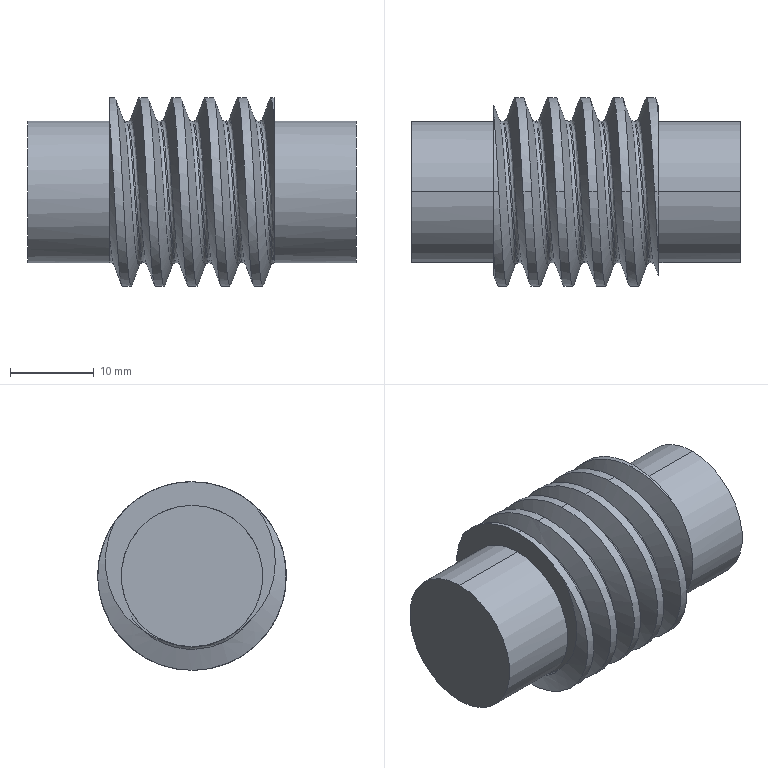Part | SolidWorks | features ICE 2, Helix 1, RefAxis 1, Revolution 1, SweepCut 1 | 1 solid | 25 faces | box 39.25 x 22.5 x 22.5 mm | volume 10547 mm3 | cylinder 16 | spline 5 | plane 4 | commonest cylinder face diameters 22.5 x12 16.875 x4